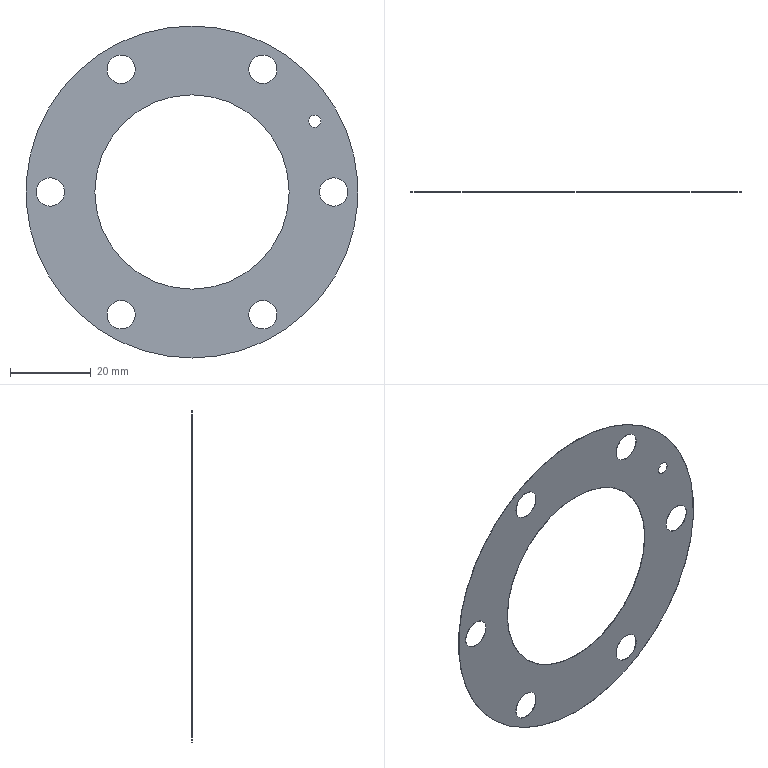Part | SolidWorks | features Extrusion 1 | 1 solid | 20 faces | box 82 x 0.1 x 82 mm | volume 323.348 mm3 | cylinder 18 | plane 2 | commonest cylinder face diameters 7 x12 3 x2 48 x2 82 x2
STEP:
#1=CARTESIAN_POINT('',(17.5,0.1,-33.811));
#2=VERTEX_POINT('',#1);
#3=CARTESIAN_POINT('',(17.5,0.1,-26.811));
#4=VERTEX_POINT('',#3);
#5=CARTESIAN_POINT('',(17.5,0.1,-30.311));
#6=DIRECTION('',(0.,1.,0.));
#7=DIRECTION('',(0.,0.,1.));
#8=AXIS2_PLACEMENT_3D('',#5,#6,#7);
#9=CIRCLE('',#8,3.5);
#10=EDGE_CURVE('',#2,#4,#9,.T.);
#11=ORIENTED_EDGE('',*,*,#10,.T.);
#12=CARTESIAN_POINT('',(17.5,0.,-26.811));
#13=VERTEX_POINT('',#12);
#14=CARTESIAN_POINT('',(17.5,0.1,-26.811));
#15=DIRECTION('',(0.,-1.,0.));
#16=VECTOR('',#15,1000.);
#17=LINE('',#14,#16);
#18=EDGE_CURVE('',#4,#13,#17,.T.);
#19=ORIENTED_EDGE('',*,*,#18,.T.);
#20=CARTESIAN_POINT('',(17.5,0.,-33.811));
#21=VERTEX_POINT('',#20);
#22=CARTESIAN_POINT('',(17.5,0.,-30.311));
#23=DIRECTION('',(0.,1.,0.));
#24=DIRECTION('',(0.,0.,1.));
#25=AXIS2_PLACEMENT_3D('',#22,#23,#24);
#26=CIRCLE('',#25,3.5);
#27=EDGE_CURVE('',#21,#13,#26,.T.);
#28=ORIENTED_EDGE('',*,*,#27,.F.);
#29=CARTESIAN_POINT('',(17.5,0.1,-33.811));
#30=DIRECTION('',(0.,-1.,0.));
#31=VECTOR('',#30,1000.);
#32=LINE('',#29,#31);
#33=EDGE_CURVE('',#2,#21,#32,.T.);
#34=ORIENTED_EDGE('',*,*,#33,.F.);
#35=EDGE_LOOP('',(#11,#19,#28,#34));
#36=FACE_OUTER_BOUND('',#35,.T.);
#37=CARTESIAN_POINT('',(17.5,0.1,-30.311));
#38=DIRECTION('',(0.,-1.,0.));
#39=DIRECTION('',(0.,0.,-1.));
#40=AXIS2_PLACEMENT_3D('',#37,#38,#39);
#41=CYLINDRICAL_SURFACE('',#40,3.5);
#42=ADVANCED_FACE('',(#36),#41,.F.);
#43=CARTESIAN_POINT('',(-17.5,0.1,-33.811));
#44=VERTEX_POINT('',#43);
#45=CARTESIAN_POINT('',(-17.5,0.1,-26.811));
#46=VERTEX_POINT('',#45);
#47=CARTESIAN_POINT('',(-17.5,0.1,-30.311));
#48=DIRECTION('',(0.,1.,0.));
#49=DIRECTION('',(0.,0.,1.));
#50=AXIS2_PLACEMENT_3D('',#47,#48,#49);
#51=CIRCLE('',#50,3.5);
#52=EDGE_CURVE('',#44,#46,#51,.T.);
#53=ORIENTED_EDGE('',*,*,#52,.T.);
#54=CARTESIAN_POINT('',(-17.5,0.,-26.811));
#55=VERTEX_POINT('',#54);
#56=CARTESIAN_POINT('',(-17.5,0.1,-26.811));
#57=DIRECTION('',(0.,-1.,0.));
#58=VECTOR('',#57,1000.);
#59=LINE('',#56,#58);
#60=EDGE_CURVE('',#46,#55,#59,.T.);
#61=ORIENTED_EDGE('',*,*,#60,.T.);
#62=CARTESIAN_POINT('',(-17.5,0.,-33.811));
#63=VERTEX_POINT('',#62);
#64=CARTESIAN_POINT('',(-17.5,0.,-30.311));
#65=DIRECTION('',(0.,1.,0.));
#66=DIRECTION('',(0.,0.,1.));
#67=AXIS2_PLACEMENT_3D('',#64,#65,#66);
#68=CIRCLE('',#67,3.5);
#69=EDGE_CURVE('',#63,#55,#68,.T.);
#70=ORIENTED_EDGE('',*,*,#69,.F.);
#71=CARTESIAN_POINT('',(-17.5,0.1,-33.811));
#72=DIRECTION('',(0.,-1.,0.));
#73=VECTOR('',#72,1000.);
#74=LINE('',#71,#73);
#75=EDGE_CURVE('',#44,#63,#74,.T.);
#76=ORIENTED_EDGE('',*,*,#75,.F.);
#77=EDGE_LOOP('',(#53,#61,#70,#76));
#78=FACE_OUTER_BOUND('',#77,.T.);
#79=CARTESIAN_POINT('',(-17.5,0.1,-30.311));
#80=DIRECTION('',(0.,-1.,0.));
#81=DIRECTION('',(0.,0.,-1.));
#82=AXIS2_PLACEMENT_3D('',#79,#80,#81);
#83=CYLINDRICAL_SURFACE('',#82,3.5);
#84=ADVANCED_FACE('',(#78),#83,.F.);
#85=CARTESIAN_POINT('',(-35.,0.1,-3.5));
#86=VERTEX_POINT('',#85);
#87=CARTESIAN_POINT('',(-35.,0.1,3.5));
#88=VERTEX_POINT('',#87);
#89=CARTESIAN_POINT('',(-35.,0.1,0.));
#90=DIRECTION('',(0.,1.,0.));
#91=DIRECTION('',(0.,0.,1.));
#92=AXIS2_PLACEMENT_3D('',#89,#90,#91);
#93=CIRCLE('',#92,3.5);
#94=EDGE_CURVE('',#86,#88,#93,.T.);
#95=ORIENTED_EDGE('',*,*,#94,.T.);
#96=CARTESIAN_POINT('',(-35.,0.,3.5));
#97=VERTEX_POINT('',#96);
#98=CARTESIAN_POINT('',(-35.,0.1,3.5));
#99=DIRECTION('',(0.,-1.,0.));
#100=VECTOR('',#99,1000.);
#101=LINE('',#98,#100);
#102=EDGE_CURVE('',#88,#97,#101,.T.);
#103=ORIENTED_EDGE('',*,*,#102,.T.);
#104=CARTESIAN_POINT('',(-35.,0.,-3.5));
#105=VERTEX_POINT('',#104);
#106=CARTESIAN_POINT('',(-35.,0.,0.));
#107=DIRECTION('',(0.,1.,0.));
#108=DIRECTION('',(0.,0.,1.));
#109=AXIS2_PLACEMENT_3D('',#106,#107,#108);
#110=CIRCLE('',#109,3.5);
#111=EDGE_CURVE('',#105,#97,#110,.T.);
#112=ORIENTED_EDGE('',*,*,#111,.F.);
#113=CARTESIAN_POINT('',(-35.,0.1,-3.5));
#114=DIRECTION('',(0.,-1.,0.));
#115=VECTOR('',#114,1000.);
#116=LINE('',#113,#115);
#117=EDGE_CURVE('',#86,#105,#116,.T.);
#118=ORIENTED_EDGE('',*,*,#117,.F.);
#119=EDGE_LOOP('',(#95,#103,#112,#118));
#120=FACE_OUTER_BOUND('',#119,.T.);
#121=CARTESIAN_POINT('',(-35.,0.1,0.));
#122=DIRECTION('',(0.,-1.,0.));
#123=DIRECTION('',(0.,0.,-1.));
#124=AXIS2_PLACEMENT_3D('',#121,#122,#123);
#125=CYLINDRICAL_SURFACE('',#124,3.5);
#126=ADVANCED_FACE('',(#120),#125,.F.);
#127=CARTESIAN_POINT('',(-17.5,0.1,26.811));
#128=VERTEX_POINT('',#127);
#129=CARTESIAN_POINT('',(-17.5,0.1,33.811));
#130=VERTEX_POINT('',#129);
#131=CARTESIAN_POINT('',(-17.5,0.1,30.311));
#132=DIRECTION('',(0.,1.,0.));
#133=DIRECTION('',(0.,0.,1.));
#134=AXIS2_PLACEMENT_3D('',#131,#132,#133);
#135=CIRCLE('',#134,3.5);
#136=EDGE_CURVE('',#128,#130,#135,.T.);
#137=ORIENTED_EDGE('',*,*,#136,.T.);
#138=CARTESIAN_POINT('',(-17.5,0.,33.811));
#139=VERTEX_POINT('',#138);
#140=CARTESIAN_POINT('',(-17.5,0.1,33.811));
#141=DIRECTION('',(0.,-1.,0.));
#142=VECTOR('',#141,1000.);
#143=LINE('',#140,#142);
#144=EDGE_CURVE('',#130,#139,#143,.T.);
#145=ORIENTED_EDGE('',*,*,#144,.T.);
#146=CARTESIAN_POINT('',(-17.5,0.,26.811));
#147=VERTEX_POINT('',#146);
#148=CARTESIAN_POINT('',(-17.5,0.,30.311));
#149=DIRECTION('',(0.,1.,0.));
#150=DIRECTION('',(0.,0.,1.));
#151=AXIS2_PLACEMENT_3D('',#148,#149,#150);
#152=CIRCLE('',#151,3.5);
#153=EDGE_CURVE('',#147,#139,#152,.T.);
#154=ORIENTED_EDGE('',*,*,#153,.F.);
#155=CARTESIAN_POINT('',(-17.5,0.1,26.811));
#156=DIRECTION('',(0.,-1.,0.));
#157=VECTOR('',#156,1000.);
#158=LINE('',#155,#157);
#159=EDGE_CURVE('',#128,#147,#158,.T.);
#160=ORIENTED_EDGE('',*,*,#159,.F.);
#161=EDGE_LOOP('',(#137,#145,#154,#160));
#162=FACE_OUTER_BOUND('',#161,.T.);
#163=CARTESIAN_POINT('',(-17.5,0.1,30.311));
#164=DIRECTION('',(0.,-1.,0.));
#165=DIRECTION('',(0.,0.,-1.));
#166=AXIS2_PLACEMENT_3D('',#163,#164,#165);
#167=CYLINDRICAL_SURFACE('',#166,3.5);
#168=ADVANCED_FACE('',(#162),#167,.F.);
#169=CARTESIAN_POINT('',(17.5,0.1,26.811));
#170=VERTEX_POINT('',#169);
#171=CARTESIAN_POINT('',(17.5,0.1,33.811));
#172=VERTEX_POINT('',#171);
#173=CARTESIAN_POINT('',(17.5,0.1,30.311));
#174=DIRECTION('',(0.,1.,0.));
#175=DIRECTION('',(0.,0.,1.));
#176=AXIS2_PLACEMENT_3D('',#173,#174,#175);
#177=CIRCLE('',#176,3.5);
#178=EDGE_CURVE('',#170,#172,#177,.T.);
#179=ORIENTED_EDGE('',*,*,#178,.T.);
#180=CARTESIAN_POINT('',(17.5,0.,33.811));
#181=VERTEX_POINT('',#180);
#182=CARTESIAN_POINT('',(17.5,0.1,33.811));
#183=DIRECTION('',(0.,-1.,0.));
#184=VECTOR('',#183,1000.);
#185=LINE('',#182,#184);
#186=EDGE_CURVE('',#172,#181,#185,.T.);
#187=ORIENTED_EDGE('',*,*,#186,.T.);
#188=CARTESIAN_POINT('',(17.5,0.,26.811));
#189=VERTEX_POINT('',#188);
#190=CARTESIAN_POINT('',(17.5,0.,30.311));
#191=DIRECTION('',(0.,1.,0.));
#192=DIRECTION('',(0.,0.,1.));
#193=AXIS2_PLACEMENT_3D('',#190,#191,#192);
#194=CIRCLE('',#193,3.5);
#195=EDGE_CURVE('',#189,#181,#194,.T.);
#196=ORIENTED_EDGE('',*,*,#195,.F.);
#197=CARTESIAN_POINT('',(17.5,0.1,26.811));
#198=DIRECTION('',(0.,-1.,0.));
#199=VECTOR('',#198,1000.);
#200=LINE('',#197,#199);
#201=EDGE_CURVE('',#170,#189,#200,.T.);
#202=ORIENTED_EDGE('',*,*,#201,.F.);
#203=EDGE_LOOP('',(#179,#187,#196,#202));
#204=FACE_OUTER_BOUND('',#203,.T.);
#205=CARTESIAN_POINT('',(17.5,0.1,30.311));
#206=DIRECTION('',(0.,-1.,0.));
#207=DIRECTION('',(0.,0.,-1.));
#208=AXIS2_PLACEMENT_3D('',#205,#206,#207);
#209=CYLINDRICAL_SURFACE('',#208,3.5);
#210=ADVANCED_FACE('',(#204),#209,.F.);
#211=CARTESIAN_POINT('',(30.311,0.1,16.));
#212=VERTEX_POINT('',#211);
#213=CARTESIAN_POINT('',(30.311,0.1,19.));
#214=VERTEX_POINT('',#213);
#215=CARTESIAN_POINT('',(30.311,0.1,17.5));
#216=DIRECTION('',(0.,1.,0.));
#217=DIRECTION('',(0.,0.,1.));
#218=AXIS2_PLACEMENT_3D('',#215,#216,#217);
#219=CIRCLE('',#218,1.5);
#220=EDGE_CURVE('',#212,#214,#219,.T.);
#221=ORIENTED_EDGE('',*,*,#220,.T.);
#222=CARTESIAN_POINT('',(30.311,0.,19.));
#223=VERTEX_POINT('',#222);
#224=CARTESIAN_POINT('',(30.311,0.1,19.));
#225=DIRECTION('',(0.,-1.,0.));
#226=VECTOR('',#225,1000.);
#227=LINE('',#224,#226);
#228=EDGE_CURVE('',#214,#223,#227,.T.);
#229=ORIENTED_EDGE('',*,*,#228,.T.);
#230=CARTESIAN_POINT('',(30.311,0.,16.));
#231=VERTEX_POINT('',#230);
#232=CARTESIAN_POINT('',(30.311,0.,17.5));
#233=DIRECTION('',(0.,1.,0.));
#234=DIRECTION('',(0.,0.,1.));
#235=AXIS2_PLACEMENT_3D('',#232,#233,#234);
#236=CIRCLE('',#235,1.5);
#237=EDGE_CURVE('',#231,#223,#236,.T.);
#238=ORIENTED_EDGE('',*,*,#237,.F.);
#239=CARTESIAN_POINT('',(30.311,0.1,16.));
#240=DIRECTION('',(0.,-1.,0.));
#241=VECTOR('',#240,1000.);
#242=LINE('',#239,#241);
#243=EDGE_CURVE('',#212,#231,#242,.T.);
#244=ORIENTED_EDGE('',*,*,#243,.F.);
#245=EDGE_LOOP('',(#221,#229,#238,#244));
#246=FACE_OUTER_BOUND('',#245,.T.);
#247=CARTESIAN_POINT('',(30.311,0.1,17.5));
#248=DIRECTION('',(0.,-1.,0.));
#249=DIRECTION('',(0.,0.,-1.));
#250=AXIS2_PLACEMENT_3D('',#247,#248,#249);
#251=CYLINDRICAL_SURFACE('',#250,1.5);
#252=ADVANCED_FACE('',(#246),#251,.F.);
#253=CARTESIAN_POINT('',(35.,0.1,-3.5));
#254=VERTEX_POINT('',#253);
#255=CARTESIAN_POINT('',(35.,0.1,3.5));
#256=VERTEX_POINT('',#255);
#257=CARTESIAN_POINT('',(35.,0.1,0.));
#258=DIRECTION('',(0.,1.,0.));
#259=DIRECTION('',(0.,0.,1.));
#260=AXIS2_PLACEMENT_3D('',#257,#258,#259);
#261=CIRCLE('',#260,3.5);
#262=EDGE_CURVE('',#254,#256,#261,.T.);
#263=ORIENTED_EDGE('',*,*,#262,.T.);
#264=CARTESIAN_POINT('',(35.,0.,3.5));
#265=VERTEX_POINT('',#264);
#266=CARTESIAN_POINT('',(35.,0.1,3.5));
#267=DIRECTION('',(0.,-1.,0.));
#268=VECTOR('',#267,1000.);
#269=LINE('',#266,#268);
#270=EDGE_CURVE('',#256,#265,#269,.T.);
#271=ORIENTED_EDGE('',*,*,#270,.T.);
#272=CARTESIAN_POINT('',(35.,0.,-3.5));
#273=VERTEX_POINT('',#272);
#274=CARTESIAN_POINT('',(35.,0.,0.));
#275=DIRECTION('',(0.,1.,0.));
#276=DIRECTION('',(0.,0.,1.));
#277=AXIS2_PLACEMENT_3D('',#274,#275,#276);
#278=CIRCLE('',#277,3.5);
#279=EDGE_CURVE('',#273,#265,#278,.T.);
#280=ORIENTED_EDGE('',*,*,#279,.F.);
#281=CARTESIAN_POINT('',(35.,0.1,-3.5));
#282=DIRECTION('',(0.,-1.,0.));
#283=VECTOR('',#282,1000.);
#284=LINE('',#281,#283);
#285=EDGE_CURVE('',#254,#273,#284,.T.);
#286=ORIENTED_EDGE('',*,*,#285,.F.);
#287=EDGE_LOOP('',(#263,#271,#280,#286));
#288=FACE_OUTER_BOUND('',#287,.T.);
#289=CARTESIAN_POINT('',(35.,0.1,0.));
#290=DIRECTION('',(0.,-1.,0.));
#291=DIRECTION('',(0.,0.,-1.));
#292=AXIS2_PLACEMENT_3D('',#289,#290,#291);
#293=CYLINDRICAL_SURFACE('',#292,3.5);
#294=ADVANCED_FACE('',(#288),#293,.F.);
#295=CARTESIAN_POINT('',(0.,0.1,-24.));
#296=VERTEX_POINT('',#295);
#297=CARTESIAN_POINT('',(0.,0.1,24.));
#298=VERTEX_POINT('',#297);
#299=CARTESIAN_POINT('',(0.,0.1,0.));
#300=DIRECTION('',(0.,1.,0.));
#301=DIRECTION('',(0.,0.,1.));
#302=AXIS2_PLACEMENT_3D('',#299,#300,#301);
#303=CIRCLE('',#302,24.);
#304=EDGE_CURVE('',#296,#298,#303,.T.);
#305=ORIENTED_EDGE('',*,*,#304,.T.);
#306=CARTESIAN_POINT('',(0.,0.,24.));
#307=VERTEX_POINT('',#306);
#308=CARTESIAN_POINT('',(0.,0.1,24.));
#309=DIRECTION('',(0.,-1.,0.));
#310=VECTOR('',#309,1000.);
#311=LINE('',#308,#310);
#312=EDGE_CURVE('',#298,#307,#311,.T.);
#313=ORIENTED_EDGE('',*,*,#312,.T.);
#314=CARTESIAN_POINT('',(0.,0.,-24.));
#315=VERTEX_POINT('',#314);
#316=CARTESIAN_POINT('',(0.,0.,0.));
#317=DIRECTION('',(0.,1.,0.));
#318=DIRECTION('',(0.,0.,1.));
#319=AXIS2_PLACEMENT_3D('',#316,#317,#318);
#320=CIRCLE('',#319,24.);
#321=EDGE_CURVE('',#315,#307,#320,.T.);
#322=ORIENTED_EDGE('',*,*,#321,.F.);
#323=CARTESIAN_POINT('',(0.,0.1,-24.));
#324=DIRECTION('',(0.,-1.,0.));
#325=VECTOR('',#324,1000.);
#326=LINE('',#323,#325);
#327=EDGE_CURVE('',#296,#315,#326,.T.);
#328=ORIENTED_EDGE('',*,*,#327,.F.);
#329=EDGE_LOOP('',(#305,#313,#322,#328));
#330=FACE_OUTER_BOUND('',#329,.T.);
#331=CARTESIAN_POINT('',(0.,0.1,0.));
#332=DIRECTION('',(0.,-1.,0.));
#333=DIRECTION('',(0.,0.,-1.));
#334=AXIS2_PLACEMENT_3D('',#331,#332,#333);
#335=CYLINDRICAL_SURFACE('',#334,24.);
#336=ADVANCED_FACE('',(#330),#335,.F.);
#337=CARTESIAN_POINT('',(0.,0.1,41.));
#338=VERTEX_POINT('',#337);
#339=CARTESIAN_POINT('',(0.,0.1,-41.));
#340=VERTEX_POINT('',#339);
#341=CARTESIAN_POINT('',(0.,0.1,0.));
#342=DIRECTION('',(0.,1.,0.));
#343=DIRECTION('',(0.,0.,1.));
#344=AXIS2_PLACEMENT_3D('',#341,#342,#343);
#345=CIRCLE('',#344,41.);
#346=EDGE_CURVE('',#338,#340,#345,.T.);
#347=ORIENTED_EDGE('',*,*,#346,.F.);
#348=CARTESIAN_POINT('',(0.,0.,41.));
#349=VERTEX_POINT('',#348);
#350=CARTESIAN_POINT('',(0.,0.1,41.));
#351=DIRECTION('',(0.,-1.,0.));
#352=VECTOR('',#351,1000.);
#353=LINE('',#350,#352);
#354=EDGE_CURVE('',#338,#349,#353,.T.);
#355=ORIENTED_EDGE('',*,*,#354,.T.);
#356=CARTESIAN_POINT('',(0.,0.,-41.));
#357=VERTEX_POINT('',#356);
#358=CARTESIAN_POINT('',(0.,0.,0.));
#359=DIRECTION('',(0.,1.,0.));
#360=DIRECTION('',(0.,0.,1.));
#361=AXIS2_PLACEMENT_3D('',#358,#359,#360);
#362=CIRCLE('',#361,41.);
#363=EDGE_CURVE('',#349,#357,#362,.T.);
#364=ORIENTED_EDGE('',*,*,#363,.T.);
#365=CARTESIAN_POINT('',(0.,0.1,-41.));
#366=DIRECTION('',(0.,-1.,0.));
#367=VECTOR('',#366,1000.);
#368=LINE('',#365,#367);
#369=EDGE_CURVE('',#340,#357,#368,.T.);
#370=ORIENTED_EDGE('',*,*,#369,.F.);
#371=EDGE_LOOP('',(#347,#355,#364,#370));
#372=FACE_OUTER_BOUND('',#371,.T.);
#373=CARTESIAN_POINT('',(0.,0.1,0.));
#374=DIRECTION('',(0.,-1.,0.));
#375=DIRECTION('',(0.,0.,-1.));
#376=AXIS2_PLACEMENT_3D('',#373,#374,#375);
#377=CYLINDRICAL_SURFACE('',#376,41.);
#378=ADVANCED_FACE('',(#372),#377,.T.);
#379=ORIENTED_EDGE('',*,*,#52,.F.);
#380=CARTESIAN_POINT('',(-17.5,0.1,-30.311));
#381=DIRECTION('',(0.,1.,0.));
#382=DIRECTION('',(0.,0.,1.));
#383=AXIS2_PLACEMENT_3D('',#380,#381,#382);
#384=CIRCLE('',#383,3.5);
#385=EDGE_CURVE('',#46,#44,#384,.T.);
#386=ORIENTED_EDGE('',*,*,#385,.F.);
#387=EDGE_LOOP('',(#379,#386));
#388=FACE_BOUND('',#387,.T.);
#389=ORIENTED_EDGE('',*,*,#136,.F.);
#390=CARTESIAN_POINT('',(-17.5,0.1,30.311));
#391=DIRECTION('',(0.,1.,0.));
#392=DIRECTION('',(0.,0.,1.));
#393=AXIS2_PLACEMENT_3D('',#390,#391,#392);
#394=CIRCLE('',#393,3.5);
#395=EDGE_CURVE('',#130,#128,#394,.T.);
#396=ORIENTED_EDGE('',*,*,#395,.F.);
#397=EDGE_LOOP('',(#389,#396));
#398=FACE_BOUND('',#397,.T.);
#399=ORIENTED_EDGE('',*,*,#220,.F.);
#400=CARTESIAN_POINT('',(30.311,0.1,17.5));
#401=DIRECTION('',(0.,1.,0.));
#402=DIRECTION('',(0.,0.,1.));
#403=AXIS2_PLACEMENT_3D('',#400,#401,#402);
#404=CIRCLE('',#403,1.5);
#405=EDGE_CURVE('',#214,#212,#404,.T.);
#406=ORIENTED_EDGE('',*,*,#405,.F.);
#407=EDGE_LOOP('',(#399,#406));
#408=FACE_BOUND('',#407,.T.);
#409=ORIENTED_EDGE('',*,*,#304,.F.);
#410=CARTESIAN_POINT('',(0.,0.1,0.));
#411=DIRECTION('',(0.,1.,0.));
#412=DIRECTION('',(0.,0.,1.));
#413=AXIS2_PLACEMENT_3D('',#410,#411,#412);
#414=CIRCLE('',#413,24.);
#415=EDGE_CURVE('',#298,#296,#414,.T.);
#416=ORIENTED_EDGE('',*,*,#415,.F.);
#417=EDGE_LOOP('',(#409,#416));
#418=FACE_BOUND('',#417,.T.);
#419=CARTESIAN_POINT('',(0.,0.1,0.));
#420=DIRECTION('',(0.,1.,0.));
#421=DIRECTION('',(0.,0.,1.));
#422=AXIS2_PLACEMENT_3D('',#419,#420,#421);
#423=CIRCLE('',#422,41.);
#424=EDGE_CURVE('',#340,#338,#423,.T.);
#425=ORIENTED_EDGE('',*,*,#424,.T.);
#426=ORIENTED_EDGE('',*,*,#346,.T.);
#427=EDGE_LOOP('',(#425,#426));
#428=FACE_OUTER_BOUND('',#427,.T.);
#429=ORIENTED_EDGE('',*,*,#262,.F.);
#430=CARTESIAN_POINT('',(35.,0.1,0.));
#431=DIRECTION('',(0.,1.,0.));
#432=DIRECTION('',(0.,0.,1.));
#433=AXIS2_PLACEMENT_3D('',#430,#431,#432);
#434=CIRCLE('',#433,3.5);
#435=EDGE_CURVE('',#256,#254,#434,.T.);
#436=ORIENTED_EDGE('',*,*,#435,.F.);
#437=EDGE_LOOP('',(#429,#436));
#438=FACE_BOUND('',#437,.T.);
#439=ORIENTED_EDGE('',*,*,#178,.F.);
#440=CARTESIAN_POINT('',(17.5,0.1,30.311));
#441=DIRECTION('',(0.,1.,0.));
#442=DIRECTION('',(0.,0.,1.));
#443=AXIS2_PLACEMENT_3D('',#440,#441,#442);
#444=CIRCLE('',#443,3.5);
#445=EDGE_CURVE('',#172,#170,#444,.T.);
#446=ORIENTED_EDGE('',*,*,#445,.F.);
#447=EDGE_LOOP('',(#439,#446));
#448=FACE_BOUND('',#447,.T.);
#449=ORIENTED_EDGE('',*,*,#94,.F.);
#450=CARTESIAN_POINT('',(-35.,0.1,0.));
#451=DIRECTION('',(0.,1.,0.));
#452=DIRECTION('',(0.,0.,1.));
#453=AXIS2_PLACEMENT_3D('',#450,#451,#452);
#454=CIRCLE('',#453,3.5);
#455=EDGE_CURVE('',#88,#86,#454,.T.);
#456=ORIENTED_EDGE('',*,*,#455,.F.);
#457=EDGE_LOOP('',(#449,#456));
#458=FACE_BOUND('',#457,.T.);
#459=ORIENTED_EDGE('',*,*,#10,.F.);
#460=CARTESIAN_POINT('',(17.5,0.1,-30.311));
#461=DIRECTION('',(0.,1.,0.));
#462=DIRECTION('',(0.,0.,1.));
#463=AXIS2_PLACEMENT_3D('',#460,#461,#462);
#464=CIRCLE('',#463,3.5);
#465=EDGE_CURVE('',#4,#2,#464,.T.);
#466=ORIENTED_EDGE('',*,*,#465,.F.);
#467=EDGE_LOOP('',(#459,#466));
#468=FACE_BOUND('',#467,.T.);
#469=CARTESIAN_POINT('',(0.,0.1,0.));
#470=DIRECTION('',(0.,1.,0.));
#471=DIRECTION('',(0.,0.,1.));
#472=AXIS2_PLACEMENT_3D('',#469,#470,#471);
#473=PLANE('',#472);
#474=ADVANCED_FACE('',(#388,#398,#408,#418,#428,#438,#448,#458,#468),#473,.T.);
#475=CARTESIAN_POINT('',(0.,0.,0.));
#476=DIRECTION('',(0.,1.,0.));
#477=DIRECTION('',(0.,0.,1.));
#478=AXIS2_PLACEMENT_3D('',#475,#476,#477);
#479=CIRCLE('',#478,41.);
#480=EDGE_CURVE('',#357,#349,#479,.T.);
#481=ORIENTED_EDGE('',*,*,#480,.F.);
#482=ORIENTED_EDGE('',*,*,#363,.F.);
#483=EDGE_LOOP('',(#481,#482));
#484=FACE_OUTER_BOUND('',#483,.T.);
#485=ORIENTED_EDGE('',*,*,#321,.T.);
#486=CARTESIAN_POINT('',(0.,0.,0.));
#487=DIRECTION('',(0.,1.,0.));
#488=DIRECTION('',(0.,0.,1.));
#489=AXIS2_PLACEMENT_3D('',#486,#487,#488);
#490=CIRCLE('',#489,24.);
#491=EDGE_CURVE('',#307,#315,#490,.T.);
#492=ORIENTED_EDGE('',*,*,#491,.T.);
#493=EDGE_LOOP('',(#485,#492));
#494=FACE_BOUND('',#493,.T.);
#495=ORIENTED_EDGE('',*,*,#279,.T.);
#496=CARTESIAN_POINT('',(35.,0.,0.));
#497=DIRECTION('',(0.,1.,0.));
#498=DIRECTION('',(0.,0.,1.));
#499=AXIS2_PLACEMENT_3D('',#496,#497,#498);
#500=CIRCLE('',#499,3.5);
#501=EDGE_CURVE('',#265,#273,#500,.T.);
#502=ORIENTED_EDGE('',*,*,#501,.T.);
#503=EDGE_LOOP('',(#495,#502));
#504=FACE_BOUND('',#503,.T.);
#505=ORIENTED_EDGE('',*,*,#237,.T.);
#506=CARTESIAN_POINT('',(30.311,0.,17.5));
#507=DIRECTION('',(0.,1.,0.));
#508=DIRECTION('',(0.,0.,1.));
#509=AXIS2_PLACEMENT_3D('',#506,#507,#508);
#510=CIRCLE('',#509,1.5);
#511=EDGE_CURVE('',#223,#231,#510,.T.);
#512=ORIENTED_EDGE('',*,*,#511,.T.);
#513=EDGE_LOOP('',(#505,#512));
#514=FACE_BOUND('',#513,.T.);
#515=ORIENTED_EDGE('',*,*,#195,.T.);
#516=CARTESIAN_POINT('',(17.5,0.,30.311));
#517=DIRECTION('',(0.,1.,0.));
#518=DIRECTION('',(0.,0.,1.));
#519=AXIS2_PLACEMENT_3D('',#516,#517,#518);
#520=CIRCLE('',#519,3.5);
#521=EDGE_CURVE('',#181,#189,#520,.T.);
#522=ORIENTED_EDGE('',*,*,#521,.T.);
#523=EDGE_LOOP('',(#515,#522));
#524=FACE_BOUND('',#523,.T.);
#525=ORIENTED_EDGE('',*,*,#153,.T.);
#526=CARTESIAN_POINT('',(-17.5,0.,30.311));
#527=DIRECTION('',(0.,1.,0.));
#528=DIRECTION('',(0.,0.,1.));
#529=AXIS2_PLACEMENT_3D('',#526,#527,#528);
#530=CIRCLE('',#529,3.5);
#531=EDGE_CURVE('',#139,#147,#530,.T.);
#532=ORIENTED_EDGE('',*,*,#531,.T.);
#533=EDGE_LOOP('',(#525,#532));
#534=FACE_BOUND('',#533,.T.);
#535=ORIENTED_EDGE('',*,*,#111,.T.);
#536=CARTESIAN_POINT('',(-35.,0.,0.));
#537=DIRECTION('',(0.,1.,0.));
#538=DIRECTION('',(0.,0.,1.));
#539=AXIS2_PLACEMENT_3D('',#536,#537,#538);
#540=CIRCLE('',#539,3.5);
#541=EDGE_CURVE('',#97,#105,#540,.T.);
#542=ORIENTED_EDGE('',*,*,#541,.T.);
#543=EDGE_LOOP('',(#535,#542));
#544=FACE_BOUND('',#543,.T.);
#545=ORIENTED_EDGE('',*,*,#69,.T.);
#546=CARTESIAN_POINT('',(-17.5,0.,-30.311));
#547=DIRECTION('',(0.,1.,0.));
#548=DIRECTION('',(0.,0.,1.));
#549=AXIS2_PLACEMENT_3D('',#546,#547,#548);
#550=CIRCLE('',#549,3.5);
#551=EDGE_CURVE('',#55,#63,#550,.T.);
#552=ORIENTED_EDGE('',*,*,#551,.T.);
#553=EDGE_LOOP('',(#545,#552));
#554=FACE_BOUND('',#553,.T.);
#555=ORIENTED_EDGE('',*,*,#27,.T.);
#556=CARTESIAN_POINT('',(17.5,0.,-30.311));
#557=DIRECTION('',(0.,1.,0.));
#558=DIRECTION('',(0.,0.,1.));
#559=AXIS2_PLACEMENT_3D('',#556,#557,#558);
#560=CIRCLE('',#559,3.5);
#561=EDGE_CURVE('',#13,#21,#560,.T.);
#562=ORIENTED_EDGE('',*,*,#561,.T.);
#563=EDGE_LOOP('',(#555,#562));
#564=FACE_BOUND('',#563,.T.);
#565=CARTESIAN_POINT('',(0.,0.,0.));
#566=DIRECTION('',(0.,1.,0.));
#567=DIRECTION('',(0.,0.,1.));
#568=AXIS2_PLACEMENT_3D('',#565,#566,#567);
#569=PLANE('',#568);
#570=ADVANCED_FACE('',(#484,#494,#504,#514,#524,#534,#544,#554,#564),#569,.F.);
#571=ORIENTED_EDGE('',*,*,#354,.F.);
#572=ORIENTED_EDGE('',*,*,#424,.F.);
#573=ORIENTED_EDGE('',*,*,#369,.T.);
#574=ORIENTED_EDGE('',*,*,#480,.T.);
#575=EDGE_LOOP('',(#571,#572,#573,#574));
#576=FACE_OUTER_BOUND('',#575,.T.);
#577=CARTESIAN_POINT('',(0.,0.1,0.));
#578=DIRECTION('',(0.,-1.,0.));
#579=DIRECTION('',(0.,0.,-1.));
#580=AXIS2_PLACEMENT_3D('',#577,#578,#579);
#581=CYLINDRICAL_SURFACE('',#580,41.);
#582=ADVANCED_FACE('',(#576),#581,.T.);
#583=ORIENTED_EDGE('',*,*,#312,.F.);
#584=ORIENTED_EDGE('',*,*,#415,.T.);
#585=ORIENTED_EDGE('',*,*,#327,.T.);
#586=ORIENTED_EDGE('',*,*,#491,.F.);
#587=EDGE_LOOP('',(#583,#584,#585,#586));
#588=FACE_OUTER_BOUND('',#587,.T.);
#589=CARTESIAN_POINT('',(0.,0.1,0.));
#590=DIRECTION('',(0.,-1.,0.));
#591=DIRECTION('',(0.,0.,-1.));
#592=AXIS2_PLACEMENT_3D('',#589,#590,#591);
#593=CYLINDRICAL_SURFACE('',#592,24.);
#594=ADVANCED_FACE('',(#588),#593,.F.);
#595=ORIENTED_EDGE('',*,*,#270,.F.);
#596=ORIENTED_EDGE('',*,*,#435,.T.);
#597=ORIENTED_EDGE('',*,*,#285,.T.);
#598=ORIENTED_EDGE('',*,*,#501,.F.);
#599=EDGE_LOOP('',(#595,#596,#597,#598));
#600=FACE_OUTER_BOUND('',#599,.T.);
#601=CARTESIAN_POINT('',(35.,0.1,0.));
#602=DIRECTION('',(0.,-1.,0.));
#603=DIRECTION('',(0.,0.,-1.));
#604=AXIS2_PLACEMENT_3D('',#601,#602,#603);
#605=CYLINDRICAL_SURFACE('',#604,3.5);
#606=ADVANCED_FACE('',(#600),#605,.F.);
#607=ORIENTED_EDGE('',*,*,#228,.F.);
#608=ORIENTED_EDGE('',*,*,#405,.T.);
#609=ORIENTED_EDGE('',*,*,#243,.T.);
#610=ORIENTED_EDGE('',*,*,#511,.F.);
#611=EDGE_LOOP('',(#607,#608,#609,#610));
#612=FACE_OUTER_BOUND('',#611,.T.);
#613=CARTESIAN_POINT('',(30.311,0.1,17.5));
#614=DIRECTION('',(0.,-1.,0.));
#615=DIRECTION('',(0.,0.,-1.));
#616=AXIS2_PLACEMENT_3D('',#613,#614,#615);
#617=CYLINDRICAL_SURFACE('',#616,1.5);
#618=ADVANCED_FACE('',(#612),#617,.F.);
#619=ORIENTED_EDGE('',*,*,#186,.F.);
#620=ORIENTED_EDGE('',*,*,#445,.T.);
#621=ORIENTED_EDGE('',*,*,#201,.T.);
#622=ORIENTED_EDGE('',*,*,#521,.F.);
#623=EDGE_LOOP('',(#619,#620,#621,#622));
#624=FACE_OUTER_BOUND('',#623,.T.);
#625=CARTESIAN_POINT('',(17.5,0.1,30.311));
#626=DIRECTION('',(0.,-1.,0.));
#627=DIRECTION('',(0.,0.,-1.));
#628=AXIS2_PLACEMENT_3D('',#625,#626,#627);
#629=CYLINDRICAL_SURFACE('',#628,3.5);
#630=ADVANCED_FACE('',(#624),#629,.F.);
#631=ORIENTED_EDGE('',*,*,#144,.F.);
#632=ORIENTED_EDGE('',*,*,#395,.T.);
#633=ORIENTED_EDGE('',*,*,#159,.T.);
#634=ORIENTED_EDGE('',*,*,#531,.F.);
#635=EDGE_LOOP('',(#631,#632,#633,#634));
#636=FACE_OUTER_BOUND('',#635,.T.);
#637=CARTESIAN_POINT('',(-17.5,0.1,30.311));
#638=DIRECTION('',(0.,-1.,0.));
#639=DIRECTION('',(0.,0.,-1.));
#640=AXIS2_PLACEMENT_3D('',#637,#638,#639);
#641=CYLINDRICAL_SURFACE('',#640,3.5);
#642=ADVANCED_FACE('',(#636),#641,.F.);
#643=ORIENTED_EDGE('',*,*,#102,.F.);
#644=ORIENTED_EDGE('',*,*,#455,.T.);
#645=ORIENTED_EDGE('',*,*,#117,.T.);
#646=ORIENTED_EDGE('',*,*,#541,.F.);
#647=EDGE_LOOP('',(#643,#644,#645,#646));
#648=FACE_OUTER_BOUND('',#647,.T.);
#649=CARTESIAN_POINT('',(-35.,0.1,0.));
#650=DIRECTION('',(0.,-1.,0.));
#651=DIRECTION('',(0.,0.,-1.));
#652=AXIS2_PLACEMENT_3D('',#649,#650,#651);
#653=CYLINDRICAL_SURFACE('',#652,3.5);
#654=ADVANCED_FACE('',(#648),#653,.F.);
#655=ORIENTED_EDGE('',*,*,#60,.F.);
#656=ORIENTED_EDGE('',*,*,#385,.T.);
#657=ORIENTED_EDGE('',*,*,#75,.T.);
#658=ORIENTED_EDGE('',*,*,#551,.F.);
#659=EDGE_LOOP('',(#655,#656,#657,#658));
#660=FACE_OUTER_BOUND('',#659,.T.);
#661=CARTESIAN_POINT('',(-17.5,0.1,-30.311));
#662=DIRECTION('',(0.,-1.,0.));
#663=DIRECTION('',(0.,0.,-1.));
#664=AXIS2_PLACEMENT_3D('',#661,#662,#663);
#665=CYLINDRICAL_SURFACE('',#664,3.5);
#666=ADVANCED_FACE('',(#660),#665,.F.);
#667=ORIENTED_EDGE('',*,*,#18,.F.);
#668=ORIENTED_EDGE('',*,*,#465,.T.);
#669=ORIENTED_EDGE('',*,*,#33,.T.);
#670=ORIENTED_EDGE('',*,*,#561,.F.);
#671=EDGE_LOOP('',(#667,#668,#669,#670));
#672=FACE_OUTER_BOUND('',#671,.T.);
#673=CARTESIAN_POINT('',(17.5,0.1,-30.311));
#674=DIRECTION('',(0.,-1.,0.));
#675=DIRECTION('',(0.,0.,-1.));
#676=AXIS2_PLACEMENT_3D('',#673,#674,#675);
#677=CYLINDRICAL_SURFACE('',#676,3.5);
#678=ADVANCED_FACE('',(#672),#677,.F.);
#679=CLOSED_SHELL('',(#42,#84,#126,#168,#210,#252,#294,#336,#378,#474,#570,#582,#594,#606,#618,#630,#642,#654,#666,#678));
#680=MANIFOLD_SOLID_BREP('',#679);
#681=CARTESIAN_POINT('',(0.,0.,0.));
#682=DIRECTION('',(0.,0.,1.));
#683=DIRECTION('',(1.,0.,0.));
#684=AXIS2_PLACEMENT_3D('',#681,#682,#683);
#685=(LENGTH_UNIT()NAMED_UNIT(*)SI_UNIT(.MILLI.,.METRE.));
#686=UNCERTAINTY_MEASURE_WITH_UNIT(LENGTH_MEASURE(0.00001),#685,'','');
#687=(NAMED_UNIT(*)PLANE_ANGLE_UNIT()SI_UNIT($,.RADIAN.));
#688=(NAMED_UNIT(*)SI_UNIT($,.STERADIAN.)SOLID_ANGLE_UNIT());
#689=(GEOMETRIC_REPRESENTATION_CONTEXT(3)GLOBAL_UNCERTAINTY_ASSIGNED_CONTEXT((#686))GLOBAL_UNIT_ASSIGNED_CONTEXT((#685,#687,#688))REPRESENTATION_CONTEXT('',''));
#690=ADVANCED_BREP_SHAPE_REPRESENTATION('',(#680,#684),#689);